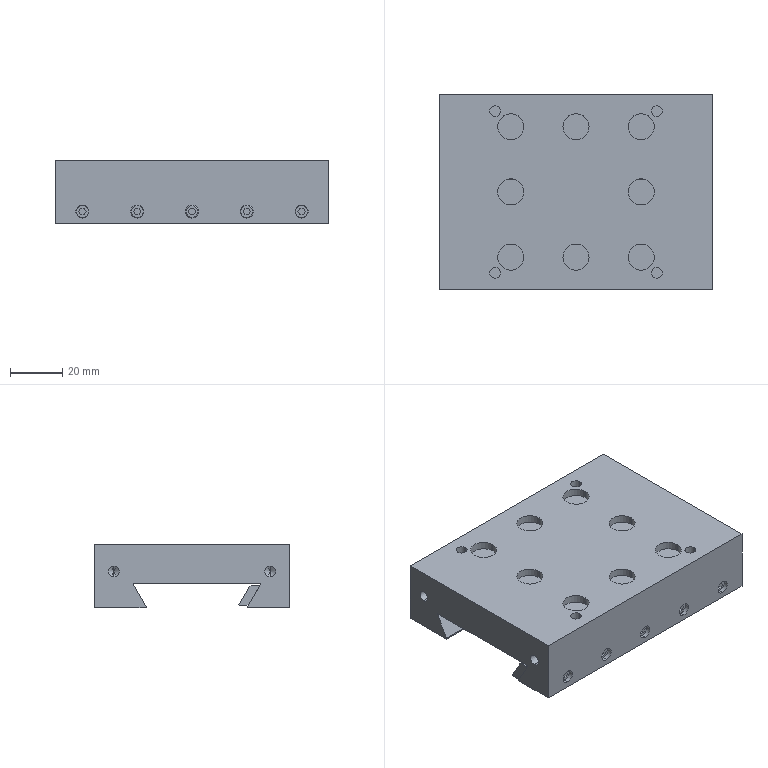Part | SolidWorks | features BaseBody 7, ICE 2 | 7 solids | 237 faces | box 105 x 75 x 24.5 mm | volume 146432 mm3 | plane 103 | cylinder 96 | cone 38 | commonest cylinder face diameters 4.134 x36 10 x36 5 x20 5.3 x4